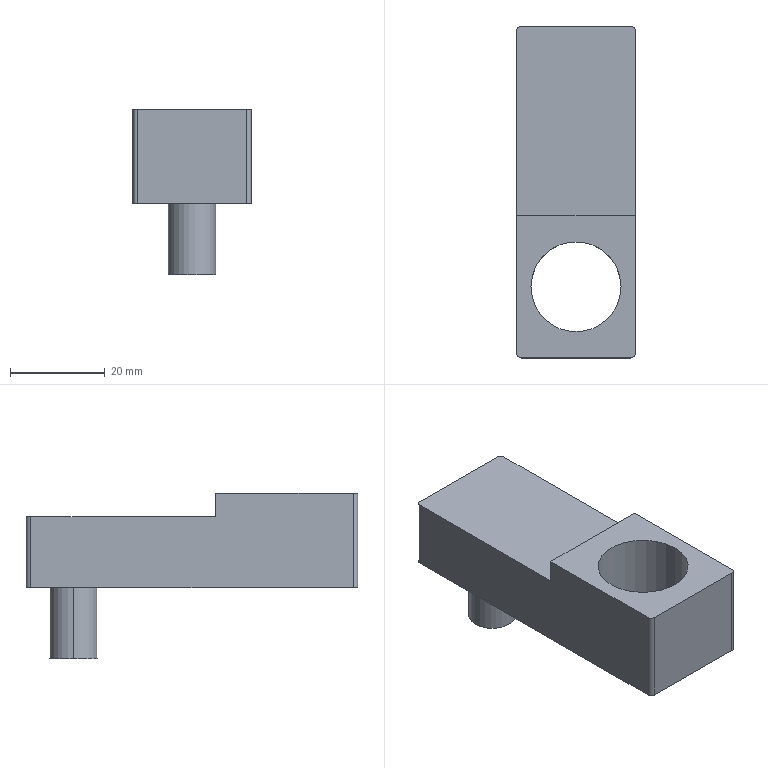Part | SolidWorks | 1 solid | 17 faces | box 25 x 70 x 35 mm | volume 25493 mm3 | plane 9 | cylinder 8 | commonest cylinder face diameters 2 x4 10 x2 19 x2
STEP:
#1=CARTESIAN_POINT('',(-5.,25.,-15.));
#2=VERTEX_POINT('',#1);
#3=CARTESIAN_POINT('',(5.,25.,-15.));
#4=VERTEX_POINT('',#3);
#5=CARTESIAN_POINT('',(0.,25.,-15.));
#6=DIRECTION('',(0.,0.,-1.));
#7=DIRECTION('',(-1.,0.,0.));
#8=AXIS2_PLACEMENT_3D('',#5,#6,#7);
#9=CIRCLE('',#8,5.);
#10=EDGE_CURVE('',#2,#4,#9,.T.);
#11=ORIENTED_EDGE('',*,*,#10,.F.);
#12=CARTESIAN_POINT('',(-5.,25.,0.));
#13=VERTEX_POINT('',#12);
#14=CARTESIAN_POINT('',(-5.,25.,-15.));
#15=DIRECTION('',(0.,0.,1.));
#16=VECTOR('',#15,1000.);
#17=LINE('',#14,#16);
#18=EDGE_CURVE('',#2,#13,#17,.T.);
#19=ORIENTED_EDGE('',*,*,#18,.T.);
#20=CARTESIAN_POINT('',(5.,25.,0.));
#21=VERTEX_POINT('',#20);
#22=CARTESIAN_POINT('',(0.,25.,0.));
#23=DIRECTION('',(0.,0.,-1.));
#24=DIRECTION('',(-1.,0.,0.));
#25=AXIS2_PLACEMENT_3D('',#22,#23,#24);
#26=CIRCLE('',#25,5.);
#27=EDGE_CURVE('',#13,#21,#26,.T.);
#28=ORIENTED_EDGE('',*,*,#27,.T.);
#29=CARTESIAN_POINT('',(5.,25.,-15.));
#30=DIRECTION('',(0.,0.,1.));
#31=VECTOR('',#30,1000.);
#32=LINE('',#29,#31);
#33=EDGE_CURVE('',#4,#21,#32,.T.);
#34=ORIENTED_EDGE('',*,*,#33,.F.);
#35=EDGE_LOOP('',(#11,#19,#28,#34));
#36=FACE_OUTER_BOUND('',#35,.T.);
#37=CARTESIAN_POINT('',(0.,25.,-15.));
#38=DIRECTION('',(0.,0.,1.));
#39=DIRECTION('',(1.,0.,0.));
#40=AXIS2_PLACEMENT_3D('',#37,#38,#39);
#41=CYLINDRICAL_SURFACE('',#40,5.);
#42=ADVANCED_FACE('',(#36),#41,.T.);
#43=CARTESIAN_POINT('',(9.5,-20.,0.));
#44=VERTEX_POINT('',#43);
#45=CARTESIAN_POINT('',(-9.5,-20.,0.));
#46=VERTEX_POINT('',#45);
#47=CARTESIAN_POINT('',(0.,-20.,0.));
#48=DIRECTION('',(0.,0.,-1.));
#49=DIRECTION('',(-1.,0.,0.));
#50=AXIS2_PLACEMENT_3D('',#47,#48,#49);
#51=CIRCLE('',#50,9.5);
#52=EDGE_CURVE('',#44,#46,#51,.T.);
#53=ORIENTED_EDGE('',*,*,#52,.T.);
#54=CARTESIAN_POINT('',(-9.5,-20.,20.));
#55=VERTEX_POINT('',#54);
#56=CARTESIAN_POINT('',(-9.5,-20.,-57.));
#57=DIRECTION('',(0.,0.,1.));
#58=VECTOR('',#57,1000.);
#59=LINE('',#56,#58);
#60=EDGE_CURVE('',#46,#55,#59,.T.);
#61=ORIENTED_EDGE('',*,*,#60,.T.);
#62=CARTESIAN_POINT('',(9.5,-20.,20.));
#63=VERTEX_POINT('',#62);
#64=CARTESIAN_POINT('',(0.,-20.,20.));
#65=DIRECTION('',(0.,0.,1.));
#66=DIRECTION('',(1.,0.,0.));
#67=AXIS2_PLACEMENT_3D('',#64,#65,#66);
#68=CIRCLE('',#67,9.5);
#69=EDGE_CURVE('',#55,#63,#68,.T.);
#70=ORIENTED_EDGE('',*,*,#69,.T.);
#71=CARTESIAN_POINT('',(9.5,-20.,-57.));
#72=DIRECTION('',(0.,0.,1.));
#73=VECTOR('',#72,1000.);
#74=LINE('',#71,#73);
#75=EDGE_CURVE('',#44,#63,#74,.T.);
#76=ORIENTED_EDGE('',*,*,#75,.F.);
#77=EDGE_LOOP('',(#53,#61,#70,#76));
#78=FACE_OUTER_BOUND('',#77,.T.);
#79=CARTESIAN_POINT('',(0.,-20.,-57.));
#80=DIRECTION('',(0.,0.,1.));
#81=DIRECTION('',(1.,0.,0.));
#82=AXIS2_PLACEMENT_3D('',#79,#80,#81);
#83=CYLINDRICAL_SURFACE('',#82,9.5);
#84=ADVANCED_FACE('',(#78),#83,.F.);
#85=CARTESIAN_POINT('',(11.5,35.,15.));
#86=VERTEX_POINT('',#85);
#87=CARTESIAN_POINT('',(-11.5,35.,15.));
#88=VERTEX_POINT('',#87);
#89=CARTESIAN_POINT('',(-12.5,35.,15.));
#90=DIRECTION('',(-1.,0.,0.));
#91=VECTOR('',#90,1000.);
#92=LINE('',#89,#91);
#93=EDGE_CURVE('',#86,#88,#92,.T.);
#94=ORIENTED_EDGE('',*,*,#93,.T.);
#95=CARTESIAN_POINT('',(-12.5,34.,15.));
#96=VERTEX_POINT('',#95);
#97=CARTESIAN_POINT('',(-11.5,34.,15.));
#98=DIRECTION('',(0.,0.,1.));
#99=DIRECTION('',(-1.,0.,0.));
#100=AXIS2_PLACEMENT_3D('',#97,#98,#99);
#101=CIRCLE('',#100,1.);
#102=EDGE_CURVE('',#88,#96,#101,.T.);
#103=ORIENTED_EDGE('',*,*,#102,.T.);
#104=CARTESIAN_POINT('',(-12.5,-5.,15.));
#105=VERTEX_POINT('',#104);
#106=CARTESIAN_POINT('',(-12.5,-35.,15.));
#107=DIRECTION('',(0.,-1.,0.));
#108=VECTOR('',#107,1000.);
#109=LINE('',#106,#108);
#110=EDGE_CURVE('',#96,#105,#109,.T.);
#111=ORIENTED_EDGE('',*,*,#110,.T.);
#112=CARTESIAN_POINT('',(12.5,-5.,15.));
#113=VERTEX_POINT('',#112);
#114=CARTESIAN_POINT('',(-12.5,-5.,15.));
#115=DIRECTION('',(-1.,0.,0.));
#116=VECTOR('',#115,1000.);
#117=LINE('',#114,#116);
#118=EDGE_CURVE('',#113,#105,#117,.T.);
#119=ORIENTED_EDGE('',*,*,#118,.F.);
#120=CARTESIAN_POINT('',(12.5,34.,15.));
#121=VERTEX_POINT('',#120);
#122=CARTESIAN_POINT('',(12.5,-35.,15.));
#123=DIRECTION('',(0.,1.,0.));
#124=VECTOR('',#123,1000.);
#125=LINE('',#122,#124);
#126=EDGE_CURVE('',#113,#121,#125,.T.);
#127=ORIENTED_EDGE('',*,*,#126,.T.);
#128=CARTESIAN_POINT('',(11.5,34.,15.));
#129=DIRECTION('',(0.,0.,1.));
#130=DIRECTION('',(-1.,0.,0.));
#131=AXIS2_PLACEMENT_3D('',#128,#129,#130);
#132=CIRCLE('',#131,1.);
#133=EDGE_CURVE('',#121,#86,#132,.T.);
#134=ORIENTED_EDGE('',*,*,#133,.T.);
#135=EDGE_LOOP('',(#94,#103,#111,#119,#127,#134));
#136=FACE_OUTER_BOUND('',#135,.T.);
#137=CARTESIAN_POINT('',(0.,0.,15.));
#138=DIRECTION('',(0.,0.,-1.));
#139=DIRECTION('',(-1.,0.,0.));
#140=AXIS2_PLACEMENT_3D('',#137,#138,#139);
#141=PLANE('',#140);
#142=ADVANCED_FACE('',(#136),#141,.F.);
#143=CARTESIAN_POINT('',(12.5,-34.,20.));
#144=VERTEX_POINT('',#143);
#145=CARTESIAN_POINT('',(12.5,-5.,20.));
#146=VERTEX_POINT('',#145);
#147=CARTESIAN_POINT('',(12.5,-35.,20.));
#148=DIRECTION('',(0.,1.,0.));
#149=VECTOR('',#148,1000.);
#150=LINE('',#147,#149);
#151=EDGE_CURVE('',#144,#146,#150,.T.);
#152=ORIENTED_EDGE('',*,*,#151,.F.);
#153=CARTESIAN_POINT('',(12.5,-34.,0.));
#154=VERTEX_POINT('',#153);
#155=CARTESIAN_POINT('',(12.5,-34.,15.));
#156=DIRECTION('',(0.,0.,-1.));
#157=VECTOR('',#156,1000.);
#158=LINE('',#155,#157);
#159=EDGE_CURVE('',#144,#154,#158,.T.);
#160=ORIENTED_EDGE('',*,*,#159,.T.);
#161=CARTESIAN_POINT('',(12.5,34.,0.));
#162=VERTEX_POINT('',#161);
#163=CARTESIAN_POINT('',(12.5,-35.,0.));
#164=DIRECTION('',(0.,1.,0.));
#165=VECTOR('',#164,1000.);
#166=LINE('',#163,#165);
#167=EDGE_CURVE('',#154,#162,#166,.T.);
#168=ORIENTED_EDGE('',*,*,#167,.T.);
#169=CARTESIAN_POINT('',(12.5,34.,15.));
#170=DIRECTION('',(0.,0.,1.));
#171=VECTOR('',#170,1000.);
#172=LINE('',#169,#171);
#173=EDGE_CURVE('',#162,#121,#172,.T.);
#174=ORIENTED_EDGE('',*,*,#173,.T.);
#175=ORIENTED_EDGE('',*,*,#126,.F.);
#176=CARTESIAN_POINT('',(12.5,-5.,20.));
#177=DIRECTION('',(0.,0.,-1.));
#178=VECTOR('',#177,1000.);
#179=LINE('',#176,#178);
#180=EDGE_CURVE('',#146,#113,#179,.T.);
#181=ORIENTED_EDGE('',*,*,#180,.F.);
#182=EDGE_LOOP('',(#152,#160,#168,#174,#175,#181));
#183=FACE_OUTER_BOUND('',#182,.T.);
#184=CARTESIAN_POINT('',(12.5,-35.,15.));
#185=DIRECTION('',(-1.,0.,0.));
#186=DIRECTION('',(0.,0.,1.));
#187=AXIS2_PLACEMENT_3D('',#184,#185,#186);
#188=PLANE('',#187);
#189=ADVANCED_FACE('',(#183),#188,.F.);
#190=CARTESIAN_POINT('',(11.5,35.,0.));
#191=VERTEX_POINT('',#190);
#192=CARTESIAN_POINT('',(-11.5,35.,0.));
#193=VERTEX_POINT('',#192);
#194=CARTESIAN_POINT('',(-12.5,35.,0.));
#195=DIRECTION('',(-1.,0.,0.));
#196=VECTOR('',#195,1000.);
#197=LINE('',#194,#196);
#198=EDGE_CURVE('',#191,#193,#197,.T.);
#199=ORIENTED_EDGE('',*,*,#198,.T.);
#200=CARTESIAN_POINT('',(-11.5,35.,15.));
#201=DIRECTION('',(0.,0.,1.));
#202=VECTOR('',#201,1000.);
#203=LINE('',#200,#202);
#204=EDGE_CURVE('',#193,#88,#203,.T.);
#205=ORIENTED_EDGE('',*,*,#204,.T.);
#206=ORIENTED_EDGE('',*,*,#93,.F.);
#207=CARTESIAN_POINT('',(11.5,35.,15.));
#208=DIRECTION('',(0.,0.,-1.));
#209=VECTOR('',#208,1000.);
#210=LINE('',#207,#209);
#211=EDGE_CURVE('',#86,#191,#210,.T.);
#212=ORIENTED_EDGE('',*,*,#211,.T.);
#213=EDGE_LOOP('',(#199,#205,#206,#212));
#214=FACE_OUTER_BOUND('',#213,.T.);
#215=CARTESIAN_POINT('',(-12.5,35.,15.));
#216=DIRECTION('',(0.,-1.,0.));
#217=DIRECTION('',(0.,0.,-1.));
#218=AXIS2_PLACEMENT_3D('',#215,#216,#217);
#219=PLANE('',#218);
#220=ADVANCED_FACE('',(#214),#219,.F.);
#221=ORIENTED_EDGE('',*,*,#110,.F.);
#222=CARTESIAN_POINT('',(-12.5,34.,0.));
#223=VERTEX_POINT('',#222);
#224=CARTESIAN_POINT('',(-12.5,34.,15.));
#225=DIRECTION('',(0.,0.,-1.));
#226=VECTOR('',#225,1000.);
#227=LINE('',#224,#226);
#228=EDGE_CURVE('',#96,#223,#227,.T.);
#229=ORIENTED_EDGE('',*,*,#228,.T.);
#230=CARTESIAN_POINT('',(-12.5,-34.,0.));
#231=VERTEX_POINT('',#230);
#232=CARTESIAN_POINT('',(-12.5,-35.,0.));
#233=DIRECTION('',(0.,-1.,0.));
#234=VECTOR('',#233,1000.);
#235=LINE('',#232,#234);
#236=EDGE_CURVE('',#223,#231,#235,.T.);
#237=ORIENTED_EDGE('',*,*,#236,.T.);
#238=CARTESIAN_POINT('',(-12.5,-34.,20.));
#239=VERTEX_POINT('',#238);
#240=CARTESIAN_POINT('',(-12.5,-34.,15.));
#241=DIRECTION('',(0.,0.,1.));
#242=VECTOR('',#241,1000.);
#243=LINE('',#240,#242);
#244=EDGE_CURVE('',#231,#239,#243,.T.);
#245=ORIENTED_EDGE('',*,*,#244,.T.);
#246=CARTESIAN_POINT('',(-12.5,-5.,20.));
#247=VERTEX_POINT('',#246);
#248=CARTESIAN_POINT('',(-12.5,-35.,20.));
#249=DIRECTION('',(0.,-1.,0.));
#250=VECTOR('',#249,1000.);
#251=LINE('',#248,#250);
#252=EDGE_CURVE('',#247,#239,#251,.T.);
#253=ORIENTED_EDGE('',*,*,#252,.F.);
#254=CARTESIAN_POINT('',(-12.5,-5.,20.));
#255=DIRECTION('',(0.,0.,-1.));
#256=VECTOR('',#255,1000.);
#257=LINE('',#254,#256);
#258=EDGE_CURVE('',#247,#105,#257,.T.);
#259=ORIENTED_EDGE('',*,*,#258,.T.);
#260=EDGE_LOOP('',(#221,#229,#237,#245,#253,#259));
#261=FACE_OUTER_BOUND('',#260,.T.);
#262=CARTESIAN_POINT('',(-12.5,-35.,15.));
#263=DIRECTION('',(1.,0.,0.));
#264=DIRECTION('',(0.,0.,-1.));
#265=AXIS2_PLACEMENT_3D('',#262,#263,#264);
#266=PLANE('',#265);
#267=ADVANCED_FACE('',(#261),#266,.F.);
#268=CARTESIAN_POINT('',(-11.5,-35.,20.));
#269=VERTEX_POINT('',#268);
#270=CARTESIAN_POINT('',(11.5,-35.,20.));
#271=VERTEX_POINT('',#270);
#272=CARTESIAN_POINT('',(-12.5,-35.,20.));
#273=DIRECTION('',(1.,0.,0.));
#274=VECTOR('',#273,1000.);
#275=LINE('',#272,#274);
#276=EDGE_CURVE('',#269,#271,#275,.T.);
#277=ORIENTED_EDGE('',*,*,#276,.F.);
#278=CARTESIAN_POINT('',(-11.5,-35.,0.));
#279=VERTEX_POINT('',#278);
#280=CARTESIAN_POINT('',(-11.5,-35.,15.));
#281=DIRECTION('',(0.,0.,-1.));
#282=VECTOR('',#281,1000.);
#283=LINE('',#280,#282);
#284=EDGE_CURVE('',#269,#279,#283,.T.);
#285=ORIENTED_EDGE('',*,*,#284,.T.);
#286=CARTESIAN_POINT('',(11.5,-35.,0.));
#287=VERTEX_POINT('',#286);
#288=CARTESIAN_POINT('',(-12.5,-35.,0.));
#289=DIRECTION('',(1.,0.,0.));
#290=VECTOR('',#289,1000.);
#291=LINE('',#288,#290);
#292=EDGE_CURVE('',#279,#287,#291,.T.);
#293=ORIENTED_EDGE('',*,*,#292,.T.);
#294=CARTESIAN_POINT('',(11.5,-35.,15.));
#295=DIRECTION('',(0.,0.,1.));
#296=VECTOR('',#295,1000.);
#297=LINE('',#294,#296);
#298=EDGE_CURVE('',#287,#271,#297,.T.);
#299=ORIENTED_EDGE('',*,*,#298,.T.);
#300=EDGE_LOOP('',(#277,#285,#293,#299));
#301=FACE_OUTER_BOUND('',#300,.T.);
#302=CARTESIAN_POINT('',(-12.5,-35.,15.));
#303=DIRECTION('',(0.,1.,0.));
#304=DIRECTION('',(0.,0.,1.));
#305=AXIS2_PLACEMENT_3D('',#302,#303,#304);
#306=PLANE('',#305);
#307=ADVANCED_FACE('',(#301),#306,.F.);
#308=CARTESIAN_POINT('',(0.,25.,0.));
#309=DIRECTION('',(0.,0.,-1.));
#310=DIRECTION('',(-1.,0.,0.));
#311=AXIS2_PLACEMENT_3D('',#308,#309,#310);
#312=CIRCLE('',#311,5.);
#313=EDGE_CURVE('',#21,#13,#312,.T.);
#314=ORIENTED_EDGE('',*,*,#313,.F.);
#315=ORIENTED_EDGE('',*,*,#27,.F.);
#316=EDGE_LOOP('',(#314,#315));
#317=FACE_BOUND('',#316,.T.);
#318=ORIENTED_EDGE('',*,*,#52,.F.);
#319=CARTESIAN_POINT('',(0.,-20.,0.));
#320=DIRECTION('',(0.,0.,-1.));
#321=DIRECTION('',(-1.,0.,0.));
#322=AXIS2_PLACEMENT_3D('',#319,#320,#321);
#323=CIRCLE('',#322,9.5);
#324=EDGE_CURVE('',#46,#44,#323,.T.);
#325=ORIENTED_EDGE('',*,*,#324,.F.);
#326=EDGE_LOOP('',(#318,#325));
#327=FACE_BOUND('',#326,.T.);
#328=ORIENTED_EDGE('',*,*,#236,.F.);
#329=CARTESIAN_POINT('',(-11.5,34.,0.));
#330=DIRECTION('',(0.,0.,-1.));
#331=DIRECTION('',(-1.,0.,0.));
#332=AXIS2_PLACEMENT_3D('',#329,#330,#331);
#333=CIRCLE('',#332,1.);
#334=EDGE_CURVE('',#223,#193,#333,.T.);
#335=ORIENTED_EDGE('',*,*,#334,.T.);
#336=ORIENTED_EDGE('',*,*,#198,.F.);
#337=CARTESIAN_POINT('',(11.5,34.,0.));
#338=DIRECTION('',(0.,0.,-1.));
#339=DIRECTION('',(-1.,0.,0.));
#340=AXIS2_PLACEMENT_3D('',#337,#338,#339);
#341=CIRCLE('',#340,1.);
#342=EDGE_CURVE('',#191,#162,#341,.T.);
#343=ORIENTED_EDGE('',*,*,#342,.T.);
#344=ORIENTED_EDGE('',*,*,#167,.F.);
#345=CARTESIAN_POINT('',(11.5,-34.,0.));
#346=DIRECTION('',(0.,0.,-1.));
#347=DIRECTION('',(-1.,0.,0.));
#348=AXIS2_PLACEMENT_3D('',#345,#346,#347);
#349=CIRCLE('',#348,1.);
#350=EDGE_CURVE('',#154,#287,#349,.T.);
#351=ORIENTED_EDGE('',*,*,#350,.T.);
#352=ORIENTED_EDGE('',*,*,#292,.F.);
#353=CARTESIAN_POINT('',(-11.5,-34.,0.));
#354=DIRECTION('',(0.,0.,-1.));
#355=DIRECTION('',(-1.,0.,0.));
#356=AXIS2_PLACEMENT_3D('',#353,#354,#355);
#357=CIRCLE('',#356,1.);
#358=EDGE_CURVE('',#279,#231,#357,.T.);
#359=ORIENTED_EDGE('',*,*,#358,.T.);
#360=EDGE_LOOP('',(#328,#335,#336,#343,#344,#351,#352,#359));
#361=FACE_OUTER_BOUND('',#360,.T.);
#362=CARTESIAN_POINT('',(0.,0.,0.));
#363=DIRECTION('',(0.,0.,-1.));
#364=DIRECTION('',(-1.,0.,0.));
#365=AXIS2_PLACEMENT_3D('',#362,#363,#364);
#366=PLANE('',#365);
#367=ADVANCED_FACE('',(#317,#327,#361),#366,.T.);
#368=ORIENTED_EDGE('',*,*,#118,.T.);
#369=ORIENTED_EDGE('',*,*,#258,.F.);
#370=CARTESIAN_POINT('',(-12.5,-5.,20.));
#371=DIRECTION('',(-1.,0.,0.));
#372=VECTOR('',#371,1000.);
#373=LINE('',#370,#372);
#374=EDGE_CURVE('',#146,#247,#373,.T.);
#375=ORIENTED_EDGE('',*,*,#374,.F.);
#376=ORIENTED_EDGE('',*,*,#180,.T.);
#377=EDGE_LOOP('',(#368,#369,#375,#376));
#378=FACE_OUTER_BOUND('',#377,.T.);
#379=CARTESIAN_POINT('',(-12.5,-5.,20.));
#380=DIRECTION('',(0.,-1.,0.));
#381=DIRECTION('',(0.,0.,-1.));
#382=AXIS2_PLACEMENT_3D('',#379,#380,#381);
#383=PLANE('',#382);
#384=ADVANCED_FACE('',(#378),#383,.F.);
#385=CARTESIAN_POINT('',(0.,-20.,20.));
#386=DIRECTION('',(0.,0.,1.));
#387=DIRECTION('',(1.,0.,0.));
#388=AXIS2_PLACEMENT_3D('',#385,#386,#387);
#389=CIRCLE('',#388,9.5);
#390=EDGE_CURVE('',#63,#55,#389,.T.);
#391=ORIENTED_EDGE('',*,*,#390,.F.);
#392=ORIENTED_EDGE('',*,*,#69,.F.);
#393=EDGE_LOOP('',(#391,#392));
#394=FACE_BOUND('',#393,.T.);
#395=ORIENTED_EDGE('',*,*,#252,.T.);
#396=CARTESIAN_POINT('',(-11.5,-34.,20.));
#397=DIRECTION('',(0.,0.,1.));
#398=DIRECTION('',(-1.,0.,0.));
#399=AXIS2_PLACEMENT_3D('',#396,#397,#398);
#400=CIRCLE('',#399,1.);
#401=EDGE_CURVE('',#239,#269,#400,.T.);
#402=ORIENTED_EDGE('',*,*,#401,.T.);
#403=ORIENTED_EDGE('',*,*,#276,.T.);
#404=CARTESIAN_POINT('',(11.5,-34.,20.));
#405=DIRECTION('',(0.,0.,1.));
#406=DIRECTION('',(-1.,0.,0.));
#407=AXIS2_PLACEMENT_3D('',#404,#405,#406);
#408=CIRCLE('',#407,1.);
#409=EDGE_CURVE('',#271,#144,#408,.T.);
#410=ORIENTED_EDGE('',*,*,#409,.T.);
#411=ORIENTED_EDGE('',*,*,#151,.T.);
#412=ORIENTED_EDGE('',*,*,#374,.T.);
#413=EDGE_LOOP('',(#395,#402,#403,#410,#411,#412));
#414=FACE_OUTER_BOUND('',#413,.T.);
#415=CARTESIAN_POINT('',(0.,0.,20.));
#416=DIRECTION('',(0.,0.,-1.));
#417=DIRECTION('',(-1.,0.,0.));
#418=AXIS2_PLACEMENT_3D('',#415,#416,#417);
#419=PLANE('',#418);
#420=ADVANCED_FACE('',(#394,#414),#419,.F.);
#421=ORIENTED_EDGE('',*,*,#60,.F.);
#422=ORIENTED_EDGE('',*,*,#324,.T.);
#423=ORIENTED_EDGE('',*,*,#75,.T.);
#424=ORIENTED_EDGE('',*,*,#390,.T.);
#425=EDGE_LOOP('',(#421,#422,#423,#424));
#426=FACE_OUTER_BOUND('',#425,.T.);
#427=CARTESIAN_POINT('',(0.,-20.,-57.));
#428=DIRECTION('',(0.,0.,1.));
#429=DIRECTION('',(1.,0.,0.));
#430=AXIS2_PLACEMENT_3D('',#427,#428,#429);
#431=CYLINDRICAL_SURFACE('',#430,9.5);
#432=ADVANCED_FACE('',(#426),#431,.F.);
#433=ORIENTED_EDGE('',*,*,#102,.F.);
#434=ORIENTED_EDGE('',*,*,#204,.F.);
#435=ORIENTED_EDGE('',*,*,#334,.F.);
#436=ORIENTED_EDGE('',*,*,#228,.F.);
#437=EDGE_LOOP('',(#433,#434,#435,#436));
#438=FACE_OUTER_BOUND('',#437,.T.);
#439=CARTESIAN_POINT('',(-11.5,34.,15.));
#440=DIRECTION('',(0.,0.,-1.));
#441=DIRECTION('',(-1.,0.,0.));
#442=AXIS2_PLACEMENT_3D('',#439,#440,#441);
#443=CYLINDRICAL_SURFACE('',#442,1.);
#444=ADVANCED_FACE('',(#438),#443,.T.);
#445=ORIENTED_EDGE('',*,*,#401,.F.);
#446=ORIENTED_EDGE('',*,*,#244,.F.);
#447=ORIENTED_EDGE('',*,*,#358,.F.);
#448=ORIENTED_EDGE('',*,*,#284,.F.);
#449=EDGE_LOOP('',(#445,#446,#447,#448));
#450=FACE_OUTER_BOUND('',#449,.T.);
#451=CARTESIAN_POINT('',(-11.5,-34.,15.));
#452=DIRECTION('',(0.,0.,-1.));
#453=DIRECTION('',(-1.,0.,0.));
#454=AXIS2_PLACEMENT_3D('',#451,#452,#453);
#455=CYLINDRICAL_SURFACE('',#454,1.);
#456=ADVANCED_FACE('',(#450),#455,.T.);
#457=ORIENTED_EDGE('',*,*,#409,.F.);
#458=ORIENTED_EDGE('',*,*,#298,.F.);
#459=ORIENTED_EDGE('',*,*,#350,.F.);
#460=ORIENTED_EDGE('',*,*,#159,.F.);
#461=EDGE_LOOP('',(#457,#458,#459,#460));
#462=FACE_OUTER_BOUND('',#461,.T.);
#463=CARTESIAN_POINT('',(11.5,-34.,15.));
#464=DIRECTION('',(0.,0.,-1.));
#465=DIRECTION('',(-1.,0.,0.));
#466=AXIS2_PLACEMENT_3D('',#463,#464,#465);
#467=CYLINDRICAL_SURFACE('',#466,1.);
#468=ADVANCED_FACE('',(#462),#467,.T.);
#469=ORIENTED_EDGE('',*,*,#133,.F.);
#470=ORIENTED_EDGE('',*,*,#173,.F.);
#471=ORIENTED_EDGE('',*,*,#342,.F.);
#472=ORIENTED_EDGE('',*,*,#211,.F.);
#473=EDGE_LOOP('',(#469,#470,#471,#472));
#474=FACE_OUTER_BOUND('',#473,.T.);
#475=CARTESIAN_POINT('',(11.5,34.,15.));
#476=DIRECTION('',(0.,0.,-1.));
#477=DIRECTION('',(-1.,0.,0.));
#478=AXIS2_PLACEMENT_3D('',#475,#476,#477);
#479=CYLINDRICAL_SURFACE('',#478,1.);
#480=ADVANCED_FACE('',(#474),#479,.T.);
#481=ORIENTED_EDGE('',*,*,#18,.F.);
#482=CARTESIAN_POINT('',(0.,25.,-15.));
#483=DIRECTION('',(0.,0.,-1.));
#484=DIRECTION('',(-1.,0.,0.));
#485=AXIS2_PLACEMENT_3D('',#482,#483,#484);
#486=CIRCLE('',#485,5.);
#487=EDGE_CURVE('',#4,#2,#486,.T.);
#488=ORIENTED_EDGE('',*,*,#487,.F.);
#489=ORIENTED_EDGE('',*,*,#33,.T.);
#490=ORIENTED_EDGE('',*,*,#313,.T.);
#491=EDGE_LOOP('',(#481,#488,#489,#490));
#492=FACE_OUTER_BOUND('',#491,.T.);
#493=CARTESIAN_POINT('',(0.,25.,-15.));
#494=DIRECTION('',(0.,0.,1.));
#495=DIRECTION('',(1.,0.,0.));
#496=AXIS2_PLACEMENT_3D('',#493,#494,#495);
#497=CYLINDRICAL_SURFACE('',#496,5.);
#498=ADVANCED_FACE('',(#492),#497,.T.);
#499=ORIENTED_EDGE('',*,*,#487,.T.);
#500=ORIENTED_EDGE('',*,*,#10,.T.);
#501=EDGE_LOOP('',(#499,#500));
#502=FACE_OUTER_BOUND('',#501,.T.);
#503=CARTESIAN_POINT('',(0.,25.,-15.));
#504=DIRECTION('',(0.,0.,-1.));
#505=DIRECTION('',(-1.,0.,0.));
#506=AXIS2_PLACEMENT_3D('',#503,#504,#505);
#507=PLANE('',#506);
#508=ADVANCED_FACE('',(#502),#507,.T.);
#509=CLOSED_SHELL('',(#42,#84,#142,#189,#220,#267,#307,#367,#384,#420,#432,#444,#456,#468,#480,#498,#508));
#510=MANIFOLD_SOLID_BREP('',#509);
#511=CARTESIAN_POINT('',(0.,0.,0.));
#512=DIRECTION('',(0.,0.,1.));
#513=DIRECTION('',(1.,0.,0.));
#514=AXIS2_PLACEMENT_3D('',#511,#512,#513);
#515=(LENGTH_UNIT()NAMED_UNIT(*)SI_UNIT(.MILLI.,.METRE.));
#516=UNCERTAINTY_MEASURE_WITH_UNIT(LENGTH_MEASURE(0.00001),#515,'','');
#517=(NAMED_UNIT(*)PLANE_ANGLE_UNIT()SI_UNIT($,.RADIAN.));
#518=(NAMED_UNIT(*)SI_UNIT($,.STERADIAN.)SOLID_ANGLE_UNIT());
#519=(GEOMETRIC_REPRESENTATION_CONTEXT(3)GLOBAL_UNCERTAINTY_ASSIGNED_CONTEXT((#516))GLOBAL_UNIT_ASSIGNED_CONTEXT((#515,#517,#518))REPRESENTATION_CONTEXT('',''));
#520=ADVANCED_BREP_SHAPE_REPRESENTATION('',(#510,#514),#519);